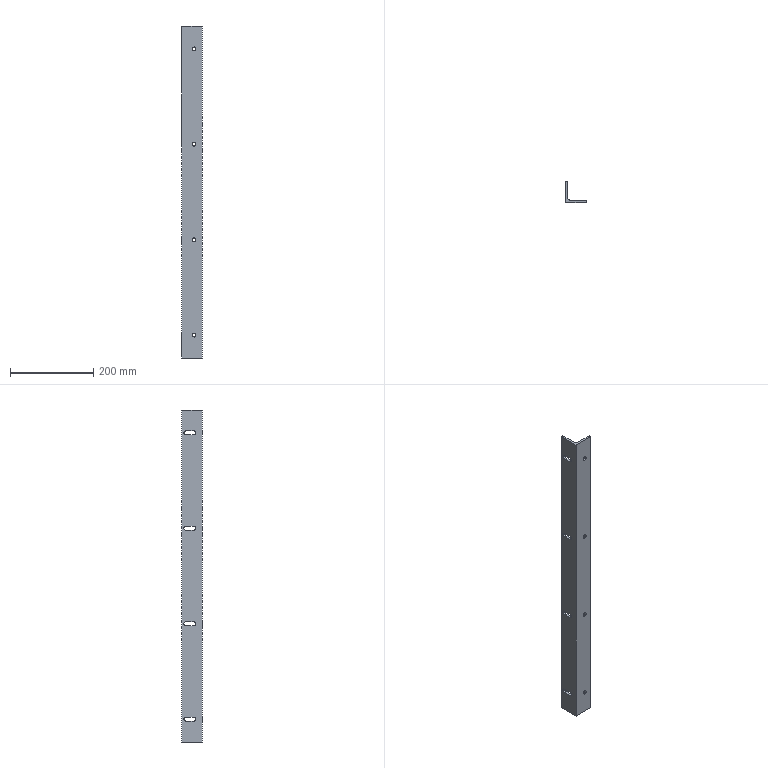Part | STEP file | 0228_203_Bracket | 1 solid | 39 faces | box 50 x 50 x 800 mm | volume 373941 mm3 | cylinder 23 | plane 16 | commonest cylinder face diameters 9 x20 7 x2 10 x1